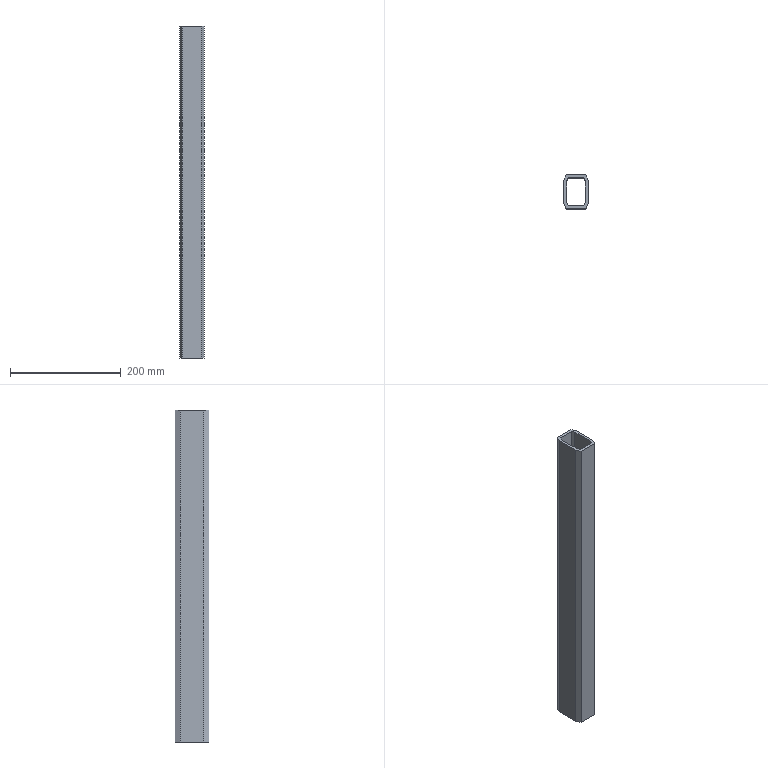Part | SolidWorks | features Extrusion 1 | 1 solid | 18 faces | box 44 x 60.7 x 600 mm | volume 534048 mm3 | plane 18
STEP:
#1=CARTESIAN_POINT('',(-17.32,136.5,600.));
#2=VERTEX_POINT('',#1);
#3=CARTESIAN_POINT('',(-22.,127.139,600.));
#4=VERTEX_POINT('',#3);
#5=CARTESIAN_POINT('',(-22.,127.139,600.));
#6=DIRECTION('',(-0.4472,-0.8944,0.));
#7=VECTOR('',#6,1000.);
#8=LINE('',#5,#7);
#9=EDGE_CURVE('',#2,#4,#8,.T.);
#10=ORIENTED_EDGE('',*,*,#9,.T.);
#11=CARTESIAN_POINT('',(-22.,85.161,600.));
#12=VERTEX_POINT('',#11);
#13=CARTESIAN_POINT('',(-22.,85.161,600.));
#14=DIRECTION('',(0.,-1.,0.));
#15=VECTOR('',#14,1000.);
#16=LINE('',#13,#15);
#17=EDGE_CURVE('',#4,#12,#16,.T.);
#18=ORIENTED_EDGE('',*,*,#17,.T.);
#19=CARTESIAN_POINT('',(-17.32,75.8,600.));
#20=VERTEX_POINT('',#19);
#21=CARTESIAN_POINT('',(-17.32,75.8,600.));
#22=DIRECTION('',(0.4472,-0.8944,0.));
#23=VECTOR('',#22,1000.);
#24=LINE('',#21,#23);
#25=EDGE_CURVE('',#12,#20,#24,.T.);
#26=ORIENTED_EDGE('',*,*,#25,.T.);
#27=CARTESIAN_POINT('',(17.32,75.8,600.));
#28=VERTEX_POINT('',#27);
#29=CARTESIAN_POINT('',(17.32,75.8,600.));
#30=DIRECTION('',(1.,0.,0.));
#31=VECTOR('',#30,1000.);
#32=LINE('',#29,#31);
#33=EDGE_CURVE('',#20,#28,#32,.T.);
#34=ORIENTED_EDGE('',*,*,#33,.T.);
#35=CARTESIAN_POINT('',(22.,85.161,600.));
#36=VERTEX_POINT('',#35);
#37=CARTESIAN_POINT('',(22.,85.161,600.));
#38=DIRECTION('',(0.4472,0.8944,0.));
#39=VECTOR('',#38,1000.);
#40=LINE('',#37,#39);
#41=EDGE_CURVE('',#28,#36,#40,.T.);
#42=ORIENTED_EDGE('',*,*,#41,.T.);
#43=CARTESIAN_POINT('',(22.,127.139,600.));
#44=VERTEX_POINT('',#43);
#45=CARTESIAN_POINT('',(22.,127.139,600.));
#46=DIRECTION('',(0.,1.,0.));
#47=VECTOR('',#46,1000.);
#48=LINE('',#45,#47);
#49=EDGE_CURVE('',#36,#44,#48,.T.);
#50=ORIENTED_EDGE('',*,*,#49,.T.);
#51=CARTESIAN_POINT('',(17.32,136.5,600.));
#52=VERTEX_POINT('',#51);
#53=CARTESIAN_POINT('',(17.32,136.5,600.));
#54=DIRECTION('',(-0.4472,0.8944,0.));
#55=VECTOR('',#54,1000.);
#56=LINE('',#53,#55);
#57=EDGE_CURVE('',#44,#52,#56,.T.);
#58=ORIENTED_EDGE('',*,*,#57,.T.);
#59=CARTESIAN_POINT('',(-17.32,136.5,600.));
#60=DIRECTION('',(-1.,0.,0.));
#61=VECTOR('',#60,1000.);
#62=LINE('',#59,#61);
#63=EDGE_CURVE('',#52,#2,#62,.T.);
#64=ORIENTED_EDGE('',*,*,#63,.T.);
#65=EDGE_LOOP('',(#10,#18,#26,#34,#42,#50,#58,#64));
#66=FACE_OUTER_BOUND('',#65,.T.);
#67=CARTESIAN_POINT('',(-14.229,131.5,600.));
#68=VERTEX_POINT('',#67);
#69=CARTESIAN_POINT('',(-17.,125.959,600.));
#70=VERTEX_POINT('',#69);
#71=CARTESIAN_POINT('',(-17.,125.959,600.));
#72=DIRECTION('',(-0.4472,-0.8944,0.));
#73=VECTOR('',#72,1000.);
#74=LINE('',#71,#73);
#75=EDGE_CURVE('',#68,#70,#74,.T.);
#76=ORIENTED_EDGE('',*,*,#75,.F.);
#77=CARTESIAN_POINT('',(14.229,131.5,600.));
#78=VERTEX_POINT('',#77);
#79=CARTESIAN_POINT('',(-14.229,131.5,600.));
#80=DIRECTION('',(-1.,0.,0.));
#81=VECTOR('',#80,1000.);
#82=LINE('',#79,#81);
#83=EDGE_CURVE('',#78,#68,#82,.T.);
#84=ORIENTED_EDGE('',*,*,#83,.F.);
#85=CARTESIAN_POINT('',(17.,125.959,600.));
#86=VERTEX_POINT('',#85);
#87=CARTESIAN_POINT('',(14.229,131.5,600.));
#88=DIRECTION('',(-0.4472,0.8944,0.));
#89=VECTOR('',#88,1000.);
#90=LINE('',#87,#89);
#91=EDGE_CURVE('',#86,#78,#90,.T.);
#92=ORIENTED_EDGE('',*,*,#91,.F.);
#93=CARTESIAN_POINT('',(17.,86.341,600.));
#94=VERTEX_POINT('',#93);
#95=CARTESIAN_POINT('',(17.,125.959,600.));
#96=DIRECTION('',(0.,1.,0.));
#97=VECTOR('',#96,1000.);
#98=LINE('',#95,#97);
#99=EDGE_CURVE('',#94,#86,#98,.T.);
#100=ORIENTED_EDGE('',*,*,#99,.F.);
#101=CARTESIAN_POINT('',(14.229,80.8,600.));
#102=VERTEX_POINT('',#101);
#103=CARTESIAN_POINT('',(17.,86.341,600.));
#104=DIRECTION('',(0.4472,0.8944,0.));
#105=VECTOR('',#104,1000.);
#106=LINE('',#103,#105);
#107=EDGE_CURVE('',#102,#94,#106,.T.);
#108=ORIENTED_EDGE('',*,*,#107,.F.);
#109=CARTESIAN_POINT('',(-14.229,80.8,600.));
#110=VERTEX_POINT('',#109);
#111=CARTESIAN_POINT('',(14.229,80.8,600.));
#112=DIRECTION('',(1.,0.,0.));
#113=VECTOR('',#112,1000.);
#114=LINE('',#111,#113);
#115=EDGE_CURVE('',#110,#102,#114,.T.);
#116=ORIENTED_EDGE('',*,*,#115,.F.);
#117=CARTESIAN_POINT('',(-17.,86.341,600.));
#118=VERTEX_POINT('',#117);
#119=CARTESIAN_POINT('',(-14.229,80.8,600.));
#120=DIRECTION('',(0.4472,-0.8944,0.));
#121=VECTOR('',#120,1000.);
#122=LINE('',#119,#121);
#123=EDGE_CURVE('',#118,#110,#122,.T.);
#124=ORIENTED_EDGE('',*,*,#123,.F.);
#125=CARTESIAN_POINT('',(-17.,86.341,600.));
#126=DIRECTION('',(0.,-1.,0.));
#127=VECTOR('',#126,1000.);
#128=LINE('',#125,#127);
#129=EDGE_CURVE('',#70,#118,#128,.T.);
#130=ORIENTED_EDGE('',*,*,#129,.F.);
#131=EDGE_LOOP('',(#76,#84,#92,#100,#108,#116,#124,#130));
#132=FACE_BOUND('',#131,.T.);
#133=CARTESIAN_POINT('',(0.,0.,600.));
#134=DIRECTION('',(0.,0.,-1.));
#135=DIRECTION('',(-1.,0.,0.));
#136=AXIS2_PLACEMENT_3D('',#133,#134,#135);
#137=PLANE('',#136);
#138=ADVANCED_FACE('',(#66,#132),#137,.F.);
#139=CARTESIAN_POINT('',(-17.32,136.5,0.));
#140=VERTEX_POINT('',#139);
#141=CARTESIAN_POINT('',(-22.,127.139,0.));
#142=VERTEX_POINT('',#141);
#143=CARTESIAN_POINT('',(-22.,127.139,0.));
#144=DIRECTION('',(-0.4472,-0.8944,0.));
#145=VECTOR('',#144,1000.);
#146=LINE('',#143,#145);
#147=EDGE_CURVE('',#140,#142,#146,.T.);
#148=ORIENTED_EDGE('',*,*,#147,.F.);
#149=CARTESIAN_POINT('',(17.32,136.5,0.));
#150=VERTEX_POINT('',#149);
#151=CARTESIAN_POINT('',(-17.32,136.5,0.));
#152=DIRECTION('',(-1.,0.,0.));
#153=VECTOR('',#152,1000.);
#154=LINE('',#151,#153);
#155=EDGE_CURVE('',#150,#140,#154,.T.);
#156=ORIENTED_EDGE('',*,*,#155,.F.);
#157=CARTESIAN_POINT('',(22.,127.139,0.));
#158=VERTEX_POINT('',#157);
#159=CARTESIAN_POINT('',(17.32,136.5,0.));
#160=DIRECTION('',(-0.4472,0.8944,0.));
#161=VECTOR('',#160,1000.);
#162=LINE('',#159,#161);
#163=EDGE_CURVE('',#158,#150,#162,.T.);
#164=ORIENTED_EDGE('',*,*,#163,.F.);
#165=CARTESIAN_POINT('',(22.,85.161,0.));
#166=VERTEX_POINT('',#165);
#167=CARTESIAN_POINT('',(22.,127.139,0.));
#168=DIRECTION('',(0.,1.,0.));
#169=VECTOR('',#168,1000.);
#170=LINE('',#167,#169);
#171=EDGE_CURVE('',#166,#158,#170,.T.);
#172=ORIENTED_EDGE('',*,*,#171,.F.);
#173=CARTESIAN_POINT('',(17.32,75.8,0.));
#174=VERTEX_POINT('',#173);
#175=CARTESIAN_POINT('',(22.,85.161,0.));
#176=DIRECTION('',(0.4472,0.8944,0.));
#177=VECTOR('',#176,1000.);
#178=LINE('',#175,#177);
#179=EDGE_CURVE('',#174,#166,#178,.T.);
#180=ORIENTED_EDGE('',*,*,#179,.F.);
#181=CARTESIAN_POINT('',(-17.32,75.8,0.));
#182=VERTEX_POINT('',#181);
#183=CARTESIAN_POINT('',(17.32,75.8,0.));
#184=DIRECTION('',(1.,0.,0.));
#185=VECTOR('',#184,1000.);
#186=LINE('',#183,#185);
#187=EDGE_CURVE('',#182,#174,#186,.T.);
#188=ORIENTED_EDGE('',*,*,#187,.F.);
#189=CARTESIAN_POINT('',(-22.,85.161,0.));
#190=VERTEX_POINT('',#189);
#191=CARTESIAN_POINT('',(-17.32,75.8,0.));
#192=DIRECTION('',(0.4472,-0.8944,0.));
#193=VECTOR('',#192,1000.);
#194=LINE('',#191,#193);
#195=EDGE_CURVE('',#190,#182,#194,.T.);
#196=ORIENTED_EDGE('',*,*,#195,.F.);
#197=CARTESIAN_POINT('',(-22.,85.161,0.));
#198=DIRECTION('',(0.,-1.,0.));
#199=VECTOR('',#198,1000.);
#200=LINE('',#197,#199);
#201=EDGE_CURVE('',#142,#190,#200,.T.);
#202=ORIENTED_EDGE('',*,*,#201,.F.);
#203=EDGE_LOOP('',(#148,#156,#164,#172,#180,#188,#196,#202));
#204=FACE_OUTER_BOUND('',#203,.T.);
#205=CARTESIAN_POINT('',(14.229,131.5,0.));
#206=VERTEX_POINT('',#205);
#207=CARTESIAN_POINT('',(-14.229,131.5,0.));
#208=VERTEX_POINT('',#207);
#209=CARTESIAN_POINT('',(-14.229,131.5,0.));
#210=DIRECTION('',(-1.,0.,0.));
#211=VECTOR('',#210,1000.);
#212=LINE('',#209,#211);
#213=EDGE_CURVE('',#206,#208,#212,.T.);
#214=ORIENTED_EDGE('',*,*,#213,.T.);
#215=CARTESIAN_POINT('',(-17.,125.959,0.));
#216=VERTEX_POINT('',#215);
#217=CARTESIAN_POINT('',(-17.,125.959,0.));
#218=DIRECTION('',(-0.4472,-0.8944,0.));
#219=VECTOR('',#218,1000.);
#220=LINE('',#217,#219);
#221=EDGE_CURVE('',#208,#216,#220,.T.);
#222=ORIENTED_EDGE('',*,*,#221,.T.);
#223=CARTESIAN_POINT('',(-17.,86.341,0.));
#224=VERTEX_POINT('',#223);
#225=CARTESIAN_POINT('',(-17.,86.341,0.));
#226=DIRECTION('',(0.,-1.,0.));
#227=VECTOR('',#226,1000.);
#228=LINE('',#225,#227);
#229=EDGE_CURVE('',#216,#224,#228,.T.);
#230=ORIENTED_EDGE('',*,*,#229,.T.);
#231=CARTESIAN_POINT('',(-14.229,80.8,0.));
#232=VERTEX_POINT('',#231);
#233=CARTESIAN_POINT('',(-14.229,80.8,0.));
#234=DIRECTION('',(0.4472,-0.8944,0.));
#235=VECTOR('',#234,1000.);
#236=LINE('',#233,#235);
#237=EDGE_CURVE('',#224,#232,#236,.T.);
#238=ORIENTED_EDGE('',*,*,#237,.T.);
#239=CARTESIAN_POINT('',(14.229,80.8,0.));
#240=VERTEX_POINT('',#239);
#241=CARTESIAN_POINT('',(14.229,80.8,0.));
#242=DIRECTION('',(1.,0.,0.));
#243=VECTOR('',#242,1000.);
#244=LINE('',#241,#243);
#245=EDGE_CURVE('',#232,#240,#244,.T.);
#246=ORIENTED_EDGE('',*,*,#245,.T.);
#247=CARTESIAN_POINT('',(17.,86.341,0.));
#248=VERTEX_POINT('',#247);
#249=CARTESIAN_POINT('',(17.,86.341,0.));
#250=DIRECTION('',(0.4472,0.8944,0.));
#251=VECTOR('',#250,1000.);
#252=LINE('',#249,#251);
#253=EDGE_CURVE('',#240,#248,#252,.T.);
#254=ORIENTED_EDGE('',*,*,#253,.T.);
#255=CARTESIAN_POINT('',(17.,125.959,0.));
#256=VERTEX_POINT('',#255);
#257=CARTESIAN_POINT('',(17.,125.959,0.));
#258=DIRECTION('',(0.,1.,0.));
#259=VECTOR('',#258,1000.);
#260=LINE('',#257,#259);
#261=EDGE_CURVE('',#248,#256,#260,.T.);
#262=ORIENTED_EDGE('',*,*,#261,.T.);
#263=CARTESIAN_POINT('',(14.229,131.5,0.));
#264=DIRECTION('',(-0.4472,0.8944,0.));
#265=VECTOR('',#264,1000.);
#266=LINE('',#263,#265);
#267=EDGE_CURVE('',#256,#206,#266,.T.);
#268=ORIENTED_EDGE('',*,*,#267,.T.);
#269=EDGE_LOOP('',(#214,#222,#230,#238,#246,#254,#262,#268));
#270=FACE_BOUND('',#269,.T.);
#271=CARTESIAN_POINT('',(0.,0.,0.));
#272=DIRECTION('',(0.,0.,-1.));
#273=DIRECTION('',(-1.,0.,0.));
#274=AXIS2_PLACEMENT_3D('',#271,#272,#273);
#275=PLANE('',#274);
#276=ADVANCED_FACE('',(#204,#270),#275,.T.);
#277=ORIENTED_EDGE('',*,*,#147,.T.);
#278=CARTESIAN_POINT('',(-22.,127.139,600.));
#279=DIRECTION('',(0.,0.,-1.));
#280=VECTOR('',#279,1000.);
#281=LINE('',#278,#280);
#282=EDGE_CURVE('',#4,#142,#281,.T.);
#283=ORIENTED_EDGE('',*,*,#282,.F.);
#284=ORIENTED_EDGE('',*,*,#9,.F.);
#285=CARTESIAN_POINT('',(-17.32,136.5,600.));
#286=DIRECTION('',(0.,0.,-1.));
#287=VECTOR('',#286,1000.);
#288=LINE('',#285,#287);
#289=EDGE_CURVE('',#2,#140,#288,.T.);
#290=ORIENTED_EDGE('',*,*,#289,.T.);
#291=EDGE_LOOP('',(#277,#283,#284,#290));
#292=FACE_OUTER_BOUND('',#291,.T.);
#293=CARTESIAN_POINT('',(-22.,127.139,600.));
#294=DIRECTION('',(0.8944,-0.4472,0.));
#295=DIRECTION('',(0.4472,0.8944,0.));
#296=AXIS2_PLACEMENT_3D('',#293,#294,#295);
#297=PLANE('',#296);
#298=ADVANCED_FACE('',(#292),#297,.F.);
#299=ORIENTED_EDGE('',*,*,#201,.T.);
#300=CARTESIAN_POINT('',(-22.,85.161,600.));
#301=DIRECTION('',(0.,0.,-1.));
#302=VECTOR('',#301,1000.);
#303=LINE('',#300,#302);
#304=EDGE_CURVE('',#12,#190,#303,.T.);
#305=ORIENTED_EDGE('',*,*,#304,.F.);
#306=ORIENTED_EDGE('',*,*,#17,.F.);
#307=ORIENTED_EDGE('',*,*,#282,.T.);
#308=EDGE_LOOP('',(#299,#305,#306,#307));
#309=FACE_OUTER_BOUND('',#308,.T.);
#310=CARTESIAN_POINT('',(-22.,85.161,600.));
#311=DIRECTION('',(1.,0.,0.));
#312=DIRECTION('',(0.,1.,0.));
#313=AXIS2_PLACEMENT_3D('',#310,#311,#312);
#314=PLANE('',#313);
#315=ADVANCED_FACE('',(#309),#314,.F.);
#316=ORIENTED_EDGE('',*,*,#195,.T.);
#317=CARTESIAN_POINT('',(-17.32,75.8,600.));
#318=DIRECTION('',(0.,0.,-1.));
#319=VECTOR('',#318,1000.);
#320=LINE('',#317,#319);
#321=EDGE_CURVE('',#20,#182,#320,.T.);
#322=ORIENTED_EDGE('',*,*,#321,.F.);
#323=ORIENTED_EDGE('',*,*,#25,.F.);
#324=ORIENTED_EDGE('',*,*,#304,.T.);
#325=EDGE_LOOP('',(#316,#322,#323,#324));
#326=FACE_OUTER_BOUND('',#325,.T.);
#327=CARTESIAN_POINT('',(-17.32,75.8,600.));
#328=DIRECTION('',(0.8944,0.4472,0.));
#329=DIRECTION('',(-0.4472,0.8944,0.));
#330=AXIS2_PLACEMENT_3D('',#327,#328,#329);
#331=PLANE('',#330);
#332=ADVANCED_FACE('',(#326),#331,.F.);
#333=ORIENTED_EDGE('',*,*,#187,.T.);
#334=CARTESIAN_POINT('',(17.32,75.8,600.));
#335=DIRECTION('',(0.,0.,-1.));
#336=VECTOR('',#335,1000.);
#337=LINE('',#334,#336);
#338=EDGE_CURVE('',#28,#174,#337,.T.);
#339=ORIENTED_EDGE('',*,*,#338,.F.);
#340=ORIENTED_EDGE('',*,*,#33,.F.);
#341=ORIENTED_EDGE('',*,*,#321,.T.);
#342=EDGE_LOOP('',(#333,#339,#340,#341));
#343=FACE_OUTER_BOUND('',#342,.T.);
#344=CARTESIAN_POINT('',(17.32,75.8,600.));
#345=DIRECTION('',(0.,1.,0.));
#346=DIRECTION('',(-1.,0.,0.));
#347=AXIS2_PLACEMENT_3D('',#344,#345,#346);
#348=PLANE('',#347);
#349=ADVANCED_FACE('',(#343),#348,.F.);
#350=ORIENTED_EDGE('',*,*,#179,.T.);
#351=CARTESIAN_POINT('',(22.,85.161,600.));
#352=DIRECTION('',(0.,0.,-1.));
#353=VECTOR('',#352,1000.);
#354=LINE('',#351,#353);
#355=EDGE_CURVE('',#36,#166,#354,.T.);
#356=ORIENTED_EDGE('',*,*,#355,.F.);
#357=ORIENTED_EDGE('',*,*,#41,.F.);
#358=ORIENTED_EDGE('',*,*,#338,.T.);
#359=EDGE_LOOP('',(#350,#356,#357,#358));
#360=FACE_OUTER_BOUND('',#359,.T.);
#361=CARTESIAN_POINT('',(22.,85.161,600.));
#362=DIRECTION('',(-0.8944,0.4472,0.));
#363=DIRECTION('',(-0.4472,-0.8944,0.));
#364=AXIS2_PLACEMENT_3D('',#361,#362,#363);
#365=PLANE('',#364);
#366=ADVANCED_FACE('',(#360),#365,.F.);
#367=ORIENTED_EDGE('',*,*,#171,.T.);
#368=CARTESIAN_POINT('',(22.,127.139,600.));
#369=DIRECTION('',(0.,0.,-1.));
#370=VECTOR('',#369,1000.);
#371=LINE('',#368,#370);
#372=EDGE_CURVE('',#44,#158,#371,.T.);
#373=ORIENTED_EDGE('',*,*,#372,.F.);
#374=ORIENTED_EDGE('',*,*,#49,.F.);
#375=ORIENTED_EDGE('',*,*,#355,.T.);
#376=EDGE_LOOP('',(#367,#373,#374,#375));
#377=FACE_OUTER_BOUND('',#376,.T.);
#378=CARTESIAN_POINT('',(22.,127.139,600.));
#379=DIRECTION('',(-1.,0.,0.));
#380=DIRECTION('',(0.,-1.,0.));
#381=AXIS2_PLACEMENT_3D('',#378,#379,#380);
#382=PLANE('',#381);
#383=ADVANCED_FACE('',(#377),#382,.F.);
#384=ORIENTED_EDGE('',*,*,#163,.T.);
#385=CARTESIAN_POINT('',(17.32,136.5,600.));
#386=DIRECTION('',(0.,0.,-1.));
#387=VECTOR('',#386,1000.);
#388=LINE('',#385,#387);
#389=EDGE_CURVE('',#52,#150,#388,.T.);
#390=ORIENTED_EDGE('',*,*,#389,.F.);
#391=ORIENTED_EDGE('',*,*,#57,.F.);
#392=ORIENTED_EDGE('',*,*,#372,.T.);
#393=EDGE_LOOP('',(#384,#390,#391,#392));
#394=FACE_OUTER_BOUND('',#393,.T.);
#395=CARTESIAN_POINT('',(17.32,136.5,600.));
#396=DIRECTION('',(-0.8944,-0.4472,0.));
#397=DIRECTION('',(0.4472,-0.8944,0.));
#398=AXIS2_PLACEMENT_3D('',#395,#396,#397);
#399=PLANE('',#398);
#400=ADVANCED_FACE('',(#394),#399,.F.);
#401=ORIENTED_EDGE('',*,*,#155,.T.);
#402=ORIENTED_EDGE('',*,*,#289,.F.);
#403=ORIENTED_EDGE('',*,*,#63,.F.);
#404=ORIENTED_EDGE('',*,*,#389,.T.);
#405=EDGE_LOOP('',(#401,#402,#403,#404));
#406=FACE_OUTER_BOUND('',#405,.T.);
#407=CARTESIAN_POINT('',(-17.32,136.5,600.));
#408=DIRECTION('',(0.,-1.,0.));
#409=DIRECTION('',(0.,0.,-1.));
#410=AXIS2_PLACEMENT_3D('',#407,#408,#409);
#411=PLANE('',#410);
#412=ADVANCED_FACE('',(#406),#411,.F.);
#413=ORIENTED_EDGE('',*,*,#221,.F.);
#414=CARTESIAN_POINT('',(-14.229,131.5,600.));
#415=DIRECTION('',(0.,0.,-1.));
#416=VECTOR('',#415,1000.);
#417=LINE('',#414,#416);
#418=EDGE_CURVE('',#68,#208,#417,.T.);
#419=ORIENTED_EDGE('',*,*,#418,.F.);
#420=ORIENTED_EDGE('',*,*,#75,.T.);
#421=CARTESIAN_POINT('',(-17.,125.959,600.));
#422=DIRECTION('',(0.,0.,-1.));
#423=VECTOR('',#422,1000.);
#424=LINE('',#421,#423);
#425=EDGE_CURVE('',#70,#216,#424,.T.);
#426=ORIENTED_EDGE('',*,*,#425,.T.);
#427=EDGE_LOOP('',(#413,#419,#420,#426));
#428=FACE_OUTER_BOUND('',#427,.T.);
#429=CARTESIAN_POINT('',(-17.,125.959,600.));
#430=DIRECTION('',(0.8944,-0.4472,0.));
#431=DIRECTION('',(0.4472,0.8944,0.));
#432=AXIS2_PLACEMENT_3D('',#429,#430,#431);
#433=PLANE('',#432);
#434=ADVANCED_FACE('',(#428),#433,.T.);
#435=ORIENTED_EDGE('',*,*,#229,.F.);
#436=ORIENTED_EDGE('',*,*,#425,.F.);
#437=ORIENTED_EDGE('',*,*,#129,.T.);
#438=CARTESIAN_POINT('',(-17.,86.341,600.));
#439=DIRECTION('',(0.,0.,-1.));
#440=VECTOR('',#439,1000.);
#441=LINE('',#438,#440);
#442=EDGE_CURVE('',#118,#224,#441,.T.);
#443=ORIENTED_EDGE('',*,*,#442,.T.);
#444=EDGE_LOOP('',(#435,#436,#437,#443));
#445=FACE_OUTER_BOUND('',#444,.T.);
#446=CARTESIAN_POINT('',(-17.,86.341,600.));
#447=DIRECTION('',(1.,0.,0.));
#448=DIRECTION('',(0.,0.,-1.));
#449=AXIS2_PLACEMENT_3D('',#446,#447,#448);
#450=PLANE('',#449);
#451=ADVANCED_FACE('',(#445),#450,.T.);
#452=ORIENTED_EDGE('',*,*,#237,.F.);
#453=ORIENTED_EDGE('',*,*,#442,.F.);
#454=ORIENTED_EDGE('',*,*,#123,.T.);
#455=CARTESIAN_POINT('',(-14.229,80.8,600.));
#456=DIRECTION('',(0.,0.,-1.));
#457=VECTOR('',#456,1000.);
#458=LINE('',#455,#457);
#459=EDGE_CURVE('',#110,#232,#458,.T.);
#460=ORIENTED_EDGE('',*,*,#459,.T.);
#461=EDGE_LOOP('',(#452,#453,#454,#460));
#462=FACE_OUTER_BOUND('',#461,.T.);
#463=CARTESIAN_POINT('',(-14.229,80.8,600.));
#464=DIRECTION('',(0.8944,0.4472,0.));
#465=DIRECTION('',(-0.4472,0.8944,0.));
#466=AXIS2_PLACEMENT_3D('',#463,#464,#465);
#467=PLANE('',#466);
#468=ADVANCED_FACE('',(#462),#467,.T.);
#469=ORIENTED_EDGE('',*,*,#245,.F.);
#470=ORIENTED_EDGE('',*,*,#459,.F.);
#471=ORIENTED_EDGE('',*,*,#115,.T.);
#472=CARTESIAN_POINT('',(14.229,80.8,600.));
#473=DIRECTION('',(0.,0.,-1.));
#474=VECTOR('',#473,1000.);
#475=LINE('',#472,#474);
#476=EDGE_CURVE('',#102,#240,#475,.T.);
#477=ORIENTED_EDGE('',*,*,#476,.T.);
#478=EDGE_LOOP('',(#469,#470,#471,#477));
#479=FACE_OUTER_BOUND('',#478,.T.);
#480=CARTESIAN_POINT('',(14.229,80.8,600.));
#481=DIRECTION('',(0.,1.,0.));
#482=DIRECTION('',(0.,0.,1.));
#483=AXIS2_PLACEMENT_3D('',#480,#481,#482);
#484=PLANE('',#483);
#485=ADVANCED_FACE('',(#479),#484,.T.);
#486=ORIENTED_EDGE('',*,*,#253,.F.);
#487=ORIENTED_EDGE('',*,*,#476,.F.);
#488=ORIENTED_EDGE('',*,*,#107,.T.);
#489=CARTESIAN_POINT('',(17.,86.341,600.));
#490=DIRECTION('',(0.,0.,-1.));
#491=VECTOR('',#490,1000.);
#492=LINE('',#489,#491);
#493=EDGE_CURVE('',#94,#248,#492,.T.);
#494=ORIENTED_EDGE('',*,*,#493,.T.);
#495=EDGE_LOOP('',(#486,#487,#488,#494));
#496=FACE_OUTER_BOUND('',#495,.T.);
#497=CARTESIAN_POINT('',(17.,86.341,600.));
#498=DIRECTION('',(-0.8944,0.4472,0.));
#499=DIRECTION('',(-0.4472,-0.8944,0.));
#500=AXIS2_PLACEMENT_3D('',#497,#498,#499);
#501=PLANE('',#500);
#502=ADVANCED_FACE('',(#496),#501,.T.);
#503=ORIENTED_EDGE('',*,*,#261,.F.);
#504=ORIENTED_EDGE('',*,*,#493,.F.);
#505=ORIENTED_EDGE('',*,*,#99,.T.);
#506=CARTESIAN_POINT('',(17.,125.959,600.));
#507=DIRECTION('',(0.,0.,-1.));
#508=VECTOR('',#507,1000.);
#509=LINE('',#506,#508);
#510=EDGE_CURVE('',#86,#256,#509,.T.);
#511=ORIENTED_EDGE('',*,*,#510,.T.);
#512=EDGE_LOOP('',(#503,#504,#505,#511));
#513=FACE_OUTER_BOUND('',#512,.T.);
#514=CARTESIAN_POINT('',(17.,125.959,600.));
#515=DIRECTION('',(-1.,0.,0.));
#516=DIRECTION('',(0.,0.,1.));
#517=AXIS2_PLACEMENT_3D('',#514,#515,#516);
#518=PLANE('',#517);
#519=ADVANCED_FACE('',(#513),#518,.T.);
#520=ORIENTED_EDGE('',*,*,#267,.F.);
#521=ORIENTED_EDGE('',*,*,#510,.F.);
#522=ORIENTED_EDGE('',*,*,#91,.T.);
#523=CARTESIAN_POINT('',(14.229,131.5,600.));
#524=DIRECTION('',(0.,0.,-1.));
#525=VECTOR('',#524,1000.);
#526=LINE('',#523,#525);
#527=EDGE_CURVE('',#78,#206,#526,.T.);
#528=ORIENTED_EDGE('',*,*,#527,.T.);
#529=EDGE_LOOP('',(#520,#521,#522,#528));
#530=FACE_OUTER_BOUND('',#529,.T.);
#531=CARTESIAN_POINT('',(14.229,131.5,600.));
#532=DIRECTION('',(-0.8944,-0.4472,0.));
#533=DIRECTION('',(0.4472,-0.8944,0.));
#534=AXIS2_PLACEMENT_3D('',#531,#532,#533);
#535=PLANE('',#534);
#536=ADVANCED_FACE('',(#530),#535,.T.);
#537=ORIENTED_EDGE('',*,*,#213,.F.);
#538=ORIENTED_EDGE('',*,*,#527,.F.);
#539=ORIENTED_EDGE('',*,*,#83,.T.);
#540=ORIENTED_EDGE('',*,*,#418,.T.);
#541=EDGE_LOOP('',(#537,#538,#539,#540));
#542=FACE_OUTER_BOUND('',#541,.T.);
#543=CARTESIAN_POINT('',(-14.229,131.5,600.));
#544=DIRECTION('',(0.,-1.,0.));
#545=DIRECTION('',(0.,0.,-1.));
#546=AXIS2_PLACEMENT_3D('',#543,#544,#545);
#547=PLANE('',#546);
#548=ADVANCED_FACE('',(#542),#547,.T.);
#549=CLOSED_SHELL('',(#138,#276,#298,#315,#332,#349,#366,#383,#400,#412,#434,#451,#468,#485,#502,#519,#536,#548));
#550=MANIFOLD_SOLID_BREP('',#549);
#551=CARTESIAN_POINT('',(0.,0.,0.));
#552=DIRECTION('',(0.,0.,1.));
#553=DIRECTION('',(1.,0.,0.));
#554=AXIS2_PLACEMENT_3D('',#551,#552,#553);
#555=(LENGTH_UNIT()NAMED_UNIT(*)SI_UNIT(.MILLI.,.METRE.));
#556=UNCERTAINTY_MEASURE_WITH_UNIT(LENGTH_MEASURE(0.00001),#555,'','');
#557=(NAMED_UNIT(*)PLANE_ANGLE_UNIT()SI_UNIT($,.RADIAN.));
#558=(NAMED_UNIT(*)SI_UNIT($,.STERADIAN.)SOLID_ANGLE_UNIT());
#559=(GEOMETRIC_REPRESENTATION_CONTEXT(3)GLOBAL_UNCERTAINTY_ASSIGNED_CONTEXT((#556))GLOBAL_UNIT_ASSIGNED_CONTEXT((#555,#557,#558))REPRESENTATION_CONTEXT('',''));
#560=ADVANCED_BREP_SHAPE_REPRESENTATION('',(#550,#554),#559);